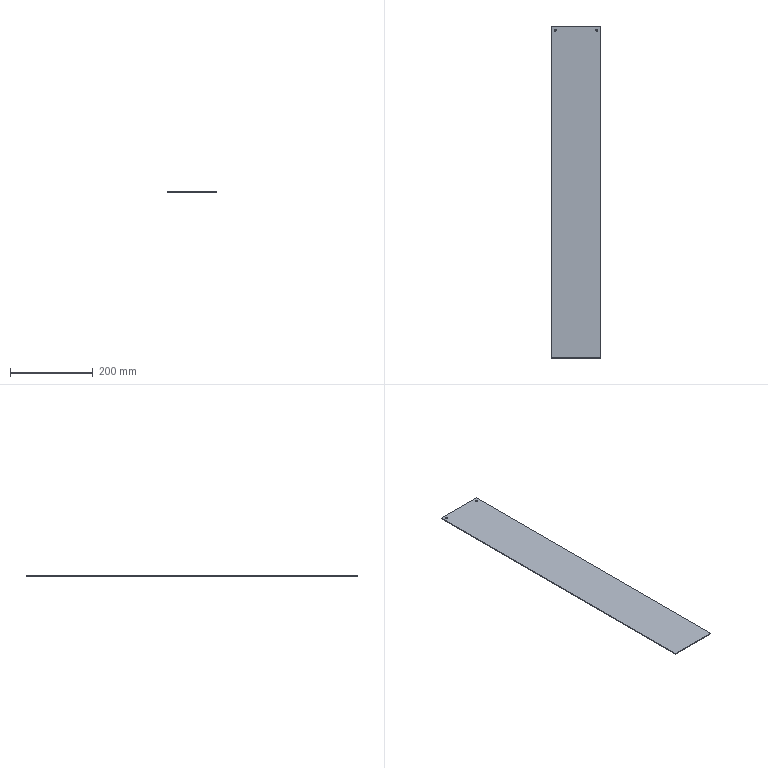Part | SolidWorks | features Extrusion 1, ICE 1 | 1 solid | 10 faces | box 120 x 800 x 2 mm | volume 191936 mm3 | plane 6 | cylinder 4 | commonest cylinder face diameters 4.5 x4
STEP:
#1=CARTESIAN_POINT('',(47.75,390.,0.));
#2=VERTEX_POINT('',#1);
#3=CARTESIAN_POINT('',(52.25,390.,0.));
#4=VERTEX_POINT('',#3);
#5=CARTESIAN_POINT('',(50.,390.,0.));
#6=DIRECTION('',(0.,0.,1.));
#7=DIRECTION('',(1.,0.,0.));
#8=AXIS2_PLACEMENT_3D('',#5,#6,#7);
#9=CIRCLE('',#8,2.25);
#10=EDGE_CURVE('',#2,#4,#9,.T.);
#11=ORIENTED_EDGE('',*,*,#10,.F.);
#12=CARTESIAN_POINT('',(47.75,390.,2.));
#13=VERTEX_POINT('',#12);
#14=CARTESIAN_POINT('',(47.75,390.,-8.));
#15=DIRECTION('',(0.,0.,1.));
#16=VECTOR('',#15,1000.);
#17=LINE('',#14,#16);
#18=EDGE_CURVE('',#2,#13,#17,.T.);
#19=ORIENTED_EDGE('',*,*,#18,.T.);
#20=CARTESIAN_POINT('',(52.25,390.,2.));
#21=VERTEX_POINT('',#20);
#22=CARTESIAN_POINT('',(50.,390.,2.));
#23=DIRECTION('',(0.,0.,1.));
#24=DIRECTION('',(1.,0.,0.));
#25=AXIS2_PLACEMENT_3D('',#22,#23,#24);
#26=CIRCLE('',#25,2.25);
#27=EDGE_CURVE('',#13,#21,#26,.T.);
#28=ORIENTED_EDGE('',*,*,#27,.T.);
#29=CARTESIAN_POINT('',(52.25,390.,-8.));
#30=DIRECTION('',(0.,0.,1.));
#31=VECTOR('',#30,1000.);
#32=LINE('',#29,#31);
#33=EDGE_CURVE('',#4,#21,#32,.T.);
#34=ORIENTED_EDGE('',*,*,#33,.F.);
#35=EDGE_LOOP('',(#11,#19,#28,#34));
#36=FACE_OUTER_BOUND('',#35,.T.);
#37=CARTESIAN_POINT('',(50.,390.,-8.));
#38=DIRECTION('',(0.,0.,1.));
#39=DIRECTION('',(1.,0.,0.));
#40=AXIS2_PLACEMENT_3D('',#37,#38,#39);
#41=CYLINDRICAL_SURFACE('',#40,2.25);
#42=ADVANCED_FACE('',(#36),#41,.F.);
#43=CARTESIAN_POINT('',(-52.25,390.,0.));
#44=VERTEX_POINT('',#43);
#45=CARTESIAN_POINT('',(-47.75,390.,0.));
#46=VERTEX_POINT('',#45);
#47=CARTESIAN_POINT('',(-50.,390.,0.));
#48=DIRECTION('',(0.,0.,1.));
#49=DIRECTION('',(1.,0.,0.));
#50=AXIS2_PLACEMENT_3D('',#47,#48,#49);
#51=CIRCLE('',#50,2.25);
#52=EDGE_CURVE('',#44,#46,#51,.T.);
#53=ORIENTED_EDGE('',*,*,#52,.F.);
#54=CARTESIAN_POINT('',(-52.25,390.,2.));
#55=VERTEX_POINT('',#54);
#56=CARTESIAN_POINT('',(-52.25,390.,-8.));
#57=DIRECTION('',(0.,0.,1.));
#58=VECTOR('',#57,1000.);
#59=LINE('',#56,#58);
#60=EDGE_CURVE('',#44,#55,#59,.T.);
#61=ORIENTED_EDGE('',*,*,#60,.T.);
#62=CARTESIAN_POINT('',(-47.75,390.,2.));
#63=VERTEX_POINT('',#62);
#64=CARTESIAN_POINT('',(-50.,390.,2.));
#65=DIRECTION('',(0.,0.,1.));
#66=DIRECTION('',(1.,0.,0.));
#67=AXIS2_PLACEMENT_3D('',#64,#65,#66);
#68=CIRCLE('',#67,2.25);
#69=EDGE_CURVE('',#55,#63,#68,.T.);
#70=ORIENTED_EDGE('',*,*,#69,.T.);
#71=CARTESIAN_POINT('',(-47.75,390.,-8.));
#72=DIRECTION('',(0.,0.,1.));
#73=VECTOR('',#72,1000.);
#74=LINE('',#71,#73);
#75=EDGE_CURVE('',#46,#63,#74,.T.);
#76=ORIENTED_EDGE('',*,*,#75,.F.);
#77=EDGE_LOOP('',(#53,#61,#70,#76));
#78=FACE_OUTER_BOUND('',#77,.T.);
#79=CARTESIAN_POINT('',(-50.,390.,-8.));
#80=DIRECTION('',(0.,0.,1.));
#81=DIRECTION('',(1.,0.,0.));
#82=AXIS2_PLACEMENT_3D('',#79,#80,#81);
#83=CYLINDRICAL_SURFACE('',#82,2.25);
#84=ADVANCED_FACE('',(#78),#83,.F.);
#85=CARTESIAN_POINT('',(60.,-400.,0.));
#86=VERTEX_POINT('',#85);
#87=CARTESIAN_POINT('',(60.,400.,0.));
#88=VERTEX_POINT('',#87);
#89=CARTESIAN_POINT('',(60.,400.,0.));
#90=DIRECTION('',(0.,1.,0.));
#91=VECTOR('',#90,1000.);
#92=LINE('',#89,#91);
#93=EDGE_CURVE('',#86,#88,#92,.T.);
#94=ORIENTED_EDGE('',*,*,#93,.T.);
#95=CARTESIAN_POINT('',(60.,400.,2.));
#96=VERTEX_POINT('',#95);
#97=CARTESIAN_POINT('',(60.,400.,2.));
#98=DIRECTION('',(0.,0.,-1.));
#99=VECTOR('',#98,1000.);
#100=LINE('',#97,#99);
#101=EDGE_CURVE('',#96,#88,#100,.T.);
#102=ORIENTED_EDGE('',*,*,#101,.F.);
#103=CARTESIAN_POINT('',(60.,-400.,2.));
#104=VERTEX_POINT('',#103);
#105=CARTESIAN_POINT('',(60.,400.,2.));
#106=DIRECTION('',(0.,1.,0.));
#107=VECTOR('',#106,1000.);
#108=LINE('',#105,#107);
#109=EDGE_CURVE('',#104,#96,#108,.T.);
#110=ORIENTED_EDGE('',*,*,#109,.F.);
#111=CARTESIAN_POINT('',(60.,-400.,2.));
#112=DIRECTION('',(0.,0.,-1.));
#113=VECTOR('',#112,1000.);
#114=LINE('',#111,#113);
#115=EDGE_CURVE('',#104,#86,#114,.T.);
#116=ORIENTED_EDGE('',*,*,#115,.T.);
#117=EDGE_LOOP('',(#94,#102,#110,#116));
#118=FACE_OUTER_BOUND('',#117,.T.);
#119=CARTESIAN_POINT('',(60.,400.,2.));
#120=DIRECTION('',(-1.,0.,0.));
#121=DIRECTION('',(0.,0.,1.));
#122=AXIS2_PLACEMENT_3D('',#119,#120,#121);
#123=PLANE('',#122);
#124=ADVANCED_FACE('',(#118),#123,.F.);
#125=CARTESIAN_POINT('',(-60.,400.,0.));
#126=VERTEX_POINT('',#125);
#127=CARTESIAN_POINT('',(-60.,400.,0.));
#128=DIRECTION('',(-1.,0.,0.));
#129=VECTOR('',#128,1000.);
#130=LINE('',#127,#129);
#131=EDGE_CURVE('',#88,#126,#130,.T.);
#132=ORIENTED_EDGE('',*,*,#131,.T.);
#133=CARTESIAN_POINT('',(-60.,400.,2.));
#134=VERTEX_POINT('',#133);
#135=CARTESIAN_POINT('',(-60.,400.,2.));
#136=DIRECTION('',(0.,0.,-1.));
#137=VECTOR('',#136,1000.);
#138=LINE('',#135,#137);
#139=EDGE_CURVE('',#134,#126,#138,.T.);
#140=ORIENTED_EDGE('',*,*,#139,.F.);
#141=CARTESIAN_POINT('',(-60.,400.,2.));
#142=DIRECTION('',(-1.,0.,0.));
#143=VECTOR('',#142,1000.);
#144=LINE('',#141,#143);
#145=EDGE_CURVE('',#96,#134,#144,.T.);
#146=ORIENTED_EDGE('',*,*,#145,.F.);
#147=ORIENTED_EDGE('',*,*,#101,.T.);
#148=EDGE_LOOP('',(#132,#140,#146,#147));
#149=FACE_OUTER_BOUND('',#148,.T.);
#150=CARTESIAN_POINT('',(-60.,400.,2.));
#151=DIRECTION('',(0.,-1.,0.));
#152=DIRECTION('',(0.,0.,-1.));
#153=AXIS2_PLACEMENT_3D('',#150,#151,#152);
#154=PLANE('',#153);
#155=ADVANCED_FACE('',(#149),#154,.F.);
#156=CARTESIAN_POINT('',(-60.,-400.,0.));
#157=VERTEX_POINT('',#156);
#158=CARTESIAN_POINT('',(-60.,400.,0.));
#159=DIRECTION('',(0.,-1.,0.));
#160=VECTOR('',#159,1000.);
#161=LINE('',#158,#160);
#162=EDGE_CURVE('',#126,#157,#161,.T.);
#163=ORIENTED_EDGE('',*,*,#162,.T.);
#164=CARTESIAN_POINT('',(-60.,-400.,2.));
#165=VERTEX_POINT('',#164);
#166=CARTESIAN_POINT('',(-60.,-400.,2.));
#167=DIRECTION('',(0.,0.,-1.));
#168=VECTOR('',#167,1000.);
#169=LINE('',#166,#168);
#170=EDGE_CURVE('',#165,#157,#169,.T.);
#171=ORIENTED_EDGE('',*,*,#170,.F.);
#172=CARTESIAN_POINT('',(-60.,400.,2.));
#173=DIRECTION('',(0.,-1.,0.));
#174=VECTOR('',#173,1000.);
#175=LINE('',#172,#174);
#176=EDGE_CURVE('',#134,#165,#175,.T.);
#177=ORIENTED_EDGE('',*,*,#176,.F.);
#178=ORIENTED_EDGE('',*,*,#139,.T.);
#179=EDGE_LOOP('',(#163,#171,#177,#178));
#180=FACE_OUTER_BOUND('',#179,.T.);
#181=CARTESIAN_POINT('',(-60.,400.,2.));
#182=DIRECTION('',(1.,0.,0.));
#183=DIRECTION('',(0.,0.,-1.));
#184=AXIS2_PLACEMENT_3D('',#181,#182,#183);
#185=PLANE('',#184);
#186=ADVANCED_FACE('',(#180),#185,.F.);
#187=CARTESIAN_POINT('',(-60.,-400.,0.));
#188=DIRECTION('',(1.,0.,0.));
#189=VECTOR('',#188,1000.);
#190=LINE('',#187,#189);
#191=EDGE_CURVE('',#157,#86,#190,.T.);
#192=ORIENTED_EDGE('',*,*,#191,.T.);
#193=ORIENTED_EDGE('',*,*,#115,.F.);
#194=CARTESIAN_POINT('',(-60.,-400.,2.));
#195=DIRECTION('',(1.,0.,0.));
#196=VECTOR('',#195,1000.);
#197=LINE('',#194,#196);
#198=EDGE_CURVE('',#165,#104,#197,.T.);
#199=ORIENTED_EDGE('',*,*,#198,.F.);
#200=ORIENTED_EDGE('',*,*,#170,.T.);
#201=EDGE_LOOP('',(#192,#193,#199,#200));
#202=FACE_OUTER_BOUND('',#201,.T.);
#203=CARTESIAN_POINT('',(-60.,-400.,2.));
#204=DIRECTION('',(0.,1.,0.));
#205=DIRECTION('',(0.,0.,1.));
#206=AXIS2_PLACEMENT_3D('',#203,#204,#205);
#207=PLANE('',#206);
#208=ADVANCED_FACE('',(#202),#207,.F.);
#209=CARTESIAN_POINT('',(50.,390.,2.));
#210=DIRECTION('',(0.,0.,1.));
#211=DIRECTION('',(1.,0.,0.));
#212=AXIS2_PLACEMENT_3D('',#209,#210,#211);
#213=CIRCLE('',#212,2.25);
#214=EDGE_CURVE('',#21,#13,#213,.T.);
#215=ORIENTED_EDGE('',*,*,#214,.F.);
#216=ORIENTED_EDGE('',*,*,#27,.F.);
#217=EDGE_LOOP('',(#215,#216));
#218=FACE_BOUND('',#217,.T.);
#219=CARTESIAN_POINT('',(-50.,390.,2.));
#220=DIRECTION('',(0.,0.,1.));
#221=DIRECTION('',(1.,0.,0.));
#222=AXIS2_PLACEMENT_3D('',#219,#220,#221);
#223=CIRCLE('',#222,2.25);
#224=EDGE_CURVE('',#63,#55,#223,.T.);
#225=ORIENTED_EDGE('',*,*,#224,.F.);
#226=ORIENTED_EDGE('',*,*,#69,.F.);
#227=EDGE_LOOP('',(#225,#226));
#228=FACE_BOUND('',#227,.T.);
#229=ORIENTED_EDGE('',*,*,#109,.T.);
#230=ORIENTED_EDGE('',*,*,#145,.T.);
#231=ORIENTED_EDGE('',*,*,#176,.T.);
#232=ORIENTED_EDGE('',*,*,#198,.T.);
#233=EDGE_LOOP('',(#229,#230,#231,#232));
#234=FACE_OUTER_BOUND('',#233,.T.);
#235=CARTESIAN_POINT('',(0.,0.,2.));
#236=DIRECTION('',(0.,0.,1.));
#237=DIRECTION('',(1.,0.,0.));
#238=AXIS2_PLACEMENT_3D('',#235,#236,#237);
#239=PLANE('',#238);
#240=ADVANCED_FACE('',(#218,#228,#234),#239,.T.);
#241=CARTESIAN_POINT('',(50.,390.,0.));
#242=DIRECTION('',(0.,0.,1.));
#243=DIRECTION('',(1.,0.,0.));
#244=AXIS2_PLACEMENT_3D('',#241,#242,#243);
#245=CIRCLE('',#244,2.25);
#246=EDGE_CURVE('',#4,#2,#245,.T.);
#247=ORIENTED_EDGE('',*,*,#246,.T.);
#248=ORIENTED_EDGE('',*,*,#10,.T.);
#249=EDGE_LOOP('',(#247,#248));
#250=FACE_BOUND('',#249,.T.);
#251=CARTESIAN_POINT('',(-50.,390.,0.));
#252=DIRECTION('',(0.,0.,1.));
#253=DIRECTION('',(1.,0.,0.));
#254=AXIS2_PLACEMENT_3D('',#251,#252,#253);
#255=CIRCLE('',#254,2.25);
#256=EDGE_CURVE('',#46,#44,#255,.T.);
#257=ORIENTED_EDGE('',*,*,#256,.T.);
#258=ORIENTED_EDGE('',*,*,#52,.T.);
#259=EDGE_LOOP('',(#257,#258));
#260=FACE_BOUND('',#259,.T.);
#261=ORIENTED_EDGE('',*,*,#93,.F.);
#262=ORIENTED_EDGE('',*,*,#191,.F.);
#263=ORIENTED_EDGE('',*,*,#162,.F.);
#264=ORIENTED_EDGE('',*,*,#131,.F.);
#265=EDGE_LOOP('',(#261,#262,#263,#264));
#266=FACE_OUTER_BOUND('',#265,.T.);
#267=CARTESIAN_POINT('',(0.,0.,0.));
#268=DIRECTION('',(0.,0.,1.));
#269=DIRECTION('',(1.,0.,0.));
#270=AXIS2_PLACEMENT_3D('',#267,#268,#269);
#271=PLANE('',#270);
#272=ADVANCED_FACE('',(#250,#260,#266),#271,.F.);
#273=ORIENTED_EDGE('',*,*,#60,.F.);
#274=ORIENTED_EDGE('',*,*,#256,.F.);
#275=ORIENTED_EDGE('',*,*,#75,.T.);
#276=ORIENTED_EDGE('',*,*,#224,.T.);
#277=EDGE_LOOP('',(#273,#274,#275,#276));
#278=FACE_OUTER_BOUND('',#277,.T.);
#279=CARTESIAN_POINT('',(-50.,390.,-8.));
#280=DIRECTION('',(0.,0.,1.));
#281=DIRECTION('',(1.,0.,0.));
#282=AXIS2_PLACEMENT_3D('',#279,#280,#281);
#283=CYLINDRICAL_SURFACE('',#282,2.25);
#284=ADVANCED_FACE('',(#278),#283,.F.);
#285=ORIENTED_EDGE('',*,*,#18,.F.);
#286=ORIENTED_EDGE('',*,*,#246,.F.);
#287=ORIENTED_EDGE('',*,*,#33,.T.);
#288=ORIENTED_EDGE('',*,*,#214,.T.);
#289=EDGE_LOOP('',(#285,#286,#287,#288));
#290=FACE_OUTER_BOUND('',#289,.T.);
#291=CARTESIAN_POINT('',(50.,390.,-8.));
#292=DIRECTION('',(0.,0.,1.));
#293=DIRECTION('',(1.,0.,0.));
#294=AXIS2_PLACEMENT_3D('',#291,#292,#293);
#295=CYLINDRICAL_SURFACE('',#294,2.25);
#296=ADVANCED_FACE('',(#290),#295,.F.);
#297=CLOSED_SHELL('',(#42,#84,#124,#155,#186,#208,#240,#272,#284,#296));
#298=MANIFOLD_SOLID_BREP('',#297);
#299=CARTESIAN_POINT('',(0.,0.,0.));
#300=DIRECTION('',(0.,0.,1.));
#301=DIRECTION('',(1.,0.,0.));
#302=AXIS2_PLACEMENT_3D('',#299,#300,#301);
#303=(LENGTH_UNIT()NAMED_UNIT(*)SI_UNIT(.MILLI.,.METRE.));
#304=UNCERTAINTY_MEASURE_WITH_UNIT(LENGTH_MEASURE(0.00001),#303,'','');
#305=(NAMED_UNIT(*)PLANE_ANGLE_UNIT()SI_UNIT($,.RADIAN.));
#306=(NAMED_UNIT(*)SI_UNIT($,.STERADIAN.)SOLID_ANGLE_UNIT());
#307=(GEOMETRIC_REPRESENTATION_CONTEXT(3)GLOBAL_UNCERTAINTY_ASSIGNED_CONTEXT((#304))GLOBAL_UNIT_ASSIGNED_CONTEXT((#303,#305,#306))REPRESENTATION_CONTEXT('',''));
#308=ADVANCED_BREP_SHAPE_REPRESENTATION('',(#298,#302),#307);